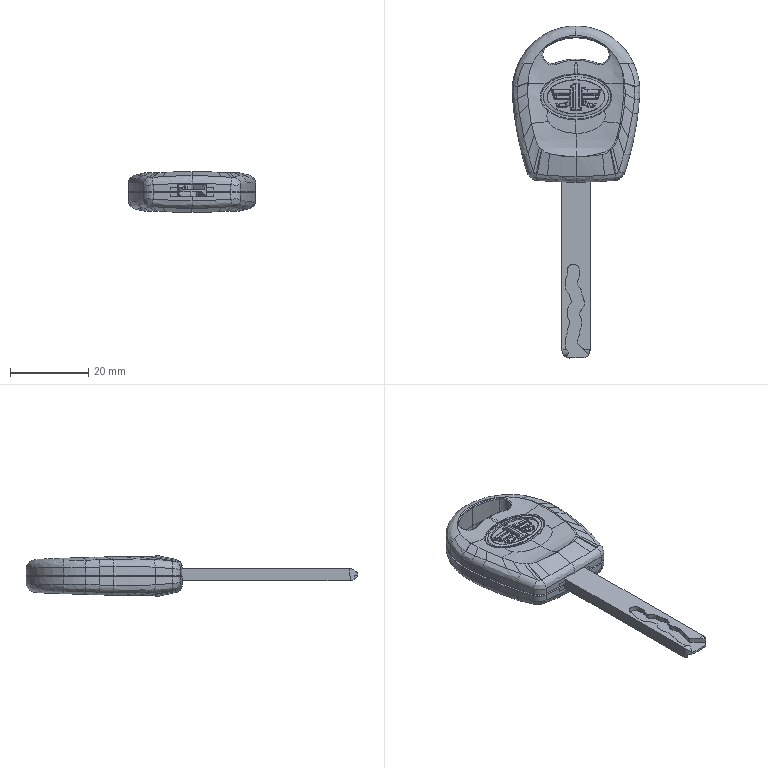Part | NX | features BREP 3 | 3 solids | 1047 faces | box 32.729 x 84.992 x 10.488 mm | volume 6335 mm3 | spline 427 | cylinder 355 | plane 181 | cone 55 | torus 27 | sphere 2 | commonest cylinder face diameters 3.1 x32 0.4 x10 2 x7 4 x6 213.872 x6 1.309 x4